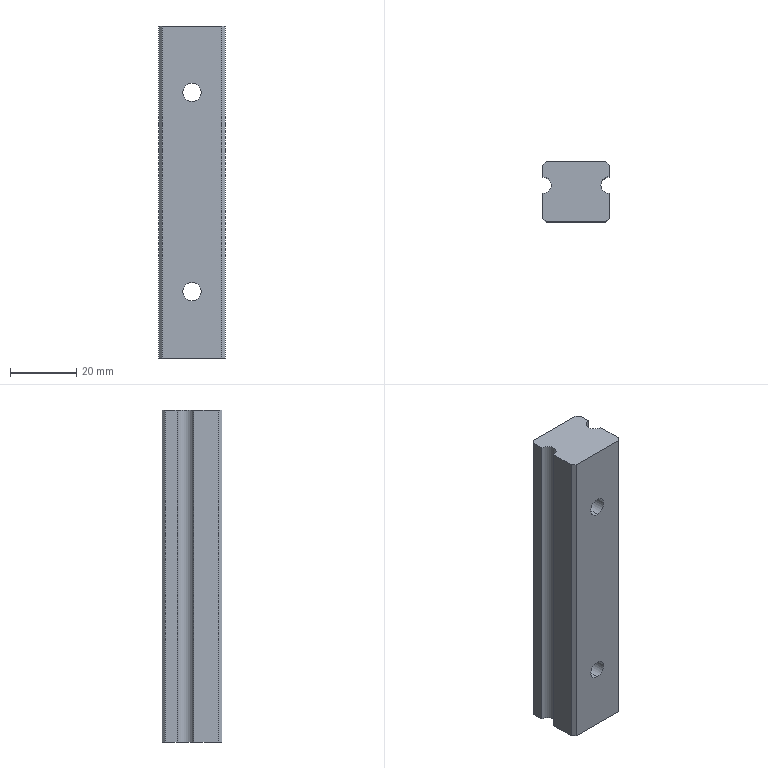Part | SolidWorks | features 3DProfileFeature 1, Extrusion 1, HoleWzd 1 | 1 solid | 25 faces | box 20 x 18 x 100 mm | volume 32357 mm3 | plane 14 | cylinder 11 | commonest cylinder face diameters 5.5 x4 10 x4 5 x3
STEP:
#1=CARTESIAN_POINT('',(10.,12.3,15.));
#2=VERTEX_POINT('',#1);
#3=CARTESIAN_POINT('',(10.,12.3,25.));
#4=VERTEX_POINT('',#3);
#5=CARTESIAN_POINT('',(10.,12.3,20.));
#6=DIRECTION('',(0.,1.,0.));
#7=DIRECTION('',(0.,0.,1.));
#8=AXIS2_PLACEMENT_3D('',#5,#6,#7);
#9=CIRCLE('',#8,5.);
#10=EDGE_CURVE('',#2,#4,#9,.T.);
#11=ORIENTED_EDGE('',*,*,#10,.F.);
#12=CARTESIAN_POINT('',(10.,18.,15.));
#13=VERTEX_POINT('',#12);
#14=CARTESIAN_POINT('',(10.,18.,15.));
#15=DIRECTION('',(0.,1.,0.));
#16=VECTOR('',#15,1000.);
#17=LINE('',#14,#16);
#18=EDGE_CURVE('',#2,#13,#17,.T.);
#19=ORIENTED_EDGE('',*,*,#18,.T.);
#20=CARTESIAN_POINT('',(10.,18.,25.));
#21=VERTEX_POINT('',#20);
#22=CARTESIAN_POINT('',(10.,18.,20.));
#23=DIRECTION('',(0.,1.,0.));
#24=DIRECTION('',(0.,0.,1.));
#25=AXIS2_PLACEMENT_3D('',#22,#23,#24);
#26=CIRCLE('',#25,5.);
#27=EDGE_CURVE('',#13,#21,#26,.T.);
#28=ORIENTED_EDGE('',*,*,#27,.T.);
#29=CARTESIAN_POINT('',(10.,18.,25.));
#30=DIRECTION('',(0.,1.,0.));
#31=VECTOR('',#30,1000.);
#32=LINE('',#29,#31);
#33=EDGE_CURVE('',#4,#21,#32,.T.);
#34=ORIENTED_EDGE('',*,*,#33,.F.);
#35=EDGE_LOOP('',(#11,#19,#28,#34));
#36=FACE_OUTER_BOUND('',#35,.T.);
#37=CARTESIAN_POINT('',(10.,18.,20.));
#38=DIRECTION('',(0.,1.,0.));
#39=DIRECTION('',(0.,0.,1.));
#40=AXIS2_PLACEMENT_3D('',#37,#38,#39);
#41=CYLINDRICAL_SURFACE('',#40,5.);
#42=ADVANCED_FACE('',(#36),#41,.F.);
#43=CARTESIAN_POINT('',(10.,0.,17.25));
#44=VERTEX_POINT('',#43);
#45=CARTESIAN_POINT('',(10.,0.,22.75));
#46=VERTEX_POINT('',#45);
#47=CARTESIAN_POINT('',(10.,0.,20.));
#48=DIRECTION('',(0.,1.,0.));
#49=DIRECTION('',(0.,0.,1.));
#50=AXIS2_PLACEMENT_3D('',#47,#48,#49);
#51=CIRCLE('',#50,2.75);
#52=EDGE_CURVE('',#44,#46,#51,.T.);
#53=ORIENTED_EDGE('',*,*,#52,.F.);
#54=CARTESIAN_POINT('',(10.,12.3,17.25));
#55=VERTEX_POINT('',#54);
#56=CARTESIAN_POINT('',(10.,18.,17.25));
#57=DIRECTION('',(0.,1.,0.));
#58=VECTOR('',#57,1000.);
#59=LINE('',#56,#58);
#60=EDGE_CURVE('',#44,#55,#59,.T.);
#61=ORIENTED_EDGE('',*,*,#60,.T.);
#62=CARTESIAN_POINT('',(10.,12.3,22.75));
#63=VERTEX_POINT('',#62);
#64=CARTESIAN_POINT('',(10.,12.3,20.));
#65=DIRECTION('',(0.,1.,0.));
#66=DIRECTION('',(0.,0.,1.));
#67=AXIS2_PLACEMENT_3D('',#64,#65,#66);
#68=CIRCLE('',#67,2.75);
#69=EDGE_CURVE('',#55,#63,#68,.T.);
#70=ORIENTED_EDGE('',*,*,#69,.T.);
#71=CARTESIAN_POINT('',(10.,18.,22.75));
#72=DIRECTION('',(0.,1.,0.));
#73=VECTOR('',#72,1000.);
#74=LINE('',#71,#73);
#75=EDGE_CURVE('',#46,#63,#74,.T.);
#76=ORIENTED_EDGE('',*,*,#75,.F.);
#77=EDGE_LOOP('',(#53,#61,#70,#76));
#78=FACE_OUTER_BOUND('',#77,.T.);
#79=CARTESIAN_POINT('',(10.,18.,20.));
#80=DIRECTION('',(0.,1.,0.));
#81=DIRECTION('',(0.,0.,1.));
#82=AXIS2_PLACEMENT_3D('',#79,#80,#81);
#83=CYLINDRICAL_SURFACE('',#82,2.75);
#84=ADVANCED_FACE('',(#78),#83,.F.);
#85=CARTESIAN_POINT('',(10.,12.3,75.));
#86=VERTEX_POINT('',#85);
#87=CARTESIAN_POINT('',(10.,12.3,85.));
#88=VERTEX_POINT('',#87);
#89=CARTESIAN_POINT('',(10.,12.3,80.));
#90=DIRECTION('',(0.,1.,0.));
#91=DIRECTION('',(0.,0.,1.));
#92=AXIS2_PLACEMENT_3D('',#89,#90,#91);
#93=CIRCLE('',#92,5.);
#94=EDGE_CURVE('',#86,#88,#93,.T.);
#95=ORIENTED_EDGE('',*,*,#94,.F.);
#96=CARTESIAN_POINT('',(10.,18.,75.));
#97=VERTEX_POINT('',#96);
#98=CARTESIAN_POINT('',(10.,18.,75.));
#99=DIRECTION('',(0.,1.,0.));
#100=VECTOR('',#99,1000.);
#101=LINE('',#98,#100);
#102=EDGE_CURVE('',#86,#97,#101,.T.);
#103=ORIENTED_EDGE('',*,*,#102,.T.);
#104=CARTESIAN_POINT('',(10.,18.,85.));
#105=VERTEX_POINT('',#104);
#106=CARTESIAN_POINT('',(10.,18.,80.));
#107=DIRECTION('',(0.,1.,0.));
#108=DIRECTION('',(0.,0.,1.));
#109=AXIS2_PLACEMENT_3D('',#106,#107,#108);
#110=CIRCLE('',#109,5.);
#111=EDGE_CURVE('',#97,#105,#110,.T.);
#112=ORIENTED_EDGE('',*,*,#111,.T.);
#113=CARTESIAN_POINT('',(10.,18.,85.));
#114=DIRECTION('',(0.,1.,0.));
#115=VECTOR('',#114,1000.);
#116=LINE('',#113,#115);
#117=EDGE_CURVE('',#88,#105,#116,.T.);
#118=ORIENTED_EDGE('',*,*,#117,.F.);
#119=EDGE_LOOP('',(#95,#103,#112,#118));
#120=FACE_OUTER_BOUND('',#119,.T.);
#121=CARTESIAN_POINT('',(10.,18.,80.));
#122=DIRECTION('',(0.,1.,0.));
#123=DIRECTION('',(0.,0.,1.));
#124=AXIS2_PLACEMENT_3D('',#121,#122,#123);
#125=CYLINDRICAL_SURFACE('',#124,5.);
#126=ADVANCED_FACE('',(#120),#125,.F.);
#127=CARTESIAN_POINT('',(10.,0.,77.25));
#128=VERTEX_POINT('',#127);
#129=CARTESIAN_POINT('',(10.,0.,82.75));
#130=VERTEX_POINT('',#129);
#131=CARTESIAN_POINT('',(10.,0.,80.));
#132=DIRECTION('',(0.,1.,0.));
#133=DIRECTION('',(0.,0.,1.));
#134=AXIS2_PLACEMENT_3D('',#131,#132,#133);
#135=CIRCLE('',#134,2.75);
#136=EDGE_CURVE('',#128,#130,#135,.T.);
#137=ORIENTED_EDGE('',*,*,#136,.F.);
#138=CARTESIAN_POINT('',(10.,12.3,77.25));
#139=VERTEX_POINT('',#138);
#140=CARTESIAN_POINT('',(10.,18.,77.25));
#141=DIRECTION('',(0.,1.,0.));
#142=VECTOR('',#141,1000.);
#143=LINE('',#140,#142);
#144=EDGE_CURVE('',#128,#139,#143,.T.);
#145=ORIENTED_EDGE('',*,*,#144,.T.);
#146=CARTESIAN_POINT('',(10.,12.3,82.75));
#147=VERTEX_POINT('',#146);
#148=CARTESIAN_POINT('',(10.,12.3,80.));
#149=DIRECTION('',(0.,1.,0.));
#150=DIRECTION('',(0.,0.,1.));
#151=AXIS2_PLACEMENT_3D('',#148,#149,#150);
#152=CIRCLE('',#151,2.75);
#153=EDGE_CURVE('',#139,#147,#152,.T.);
#154=ORIENTED_EDGE('',*,*,#153,.T.);
#155=CARTESIAN_POINT('',(10.,18.,82.75));
#156=DIRECTION('',(0.,1.,0.));
#157=VECTOR('',#156,1000.);
#158=LINE('',#155,#157);
#159=EDGE_CURVE('',#130,#147,#158,.T.);
#160=ORIENTED_EDGE('',*,*,#159,.F.);
#161=EDGE_LOOP('',(#137,#145,#154,#160));
#162=FACE_OUTER_BOUND('',#161,.T.);
#163=CARTESIAN_POINT('',(10.,18.,80.));
#164=DIRECTION('',(0.,1.,0.));
#165=DIRECTION('',(0.,0.,1.));
#166=AXIS2_PLACEMENT_3D('',#163,#164,#165);
#167=CYLINDRICAL_SURFACE('',#166,2.75);
#168=ADVANCED_FACE('',(#162),#167,.F.);
#169=CARTESIAN_POINT('',(17.5,11.,100.));
#170=VERTEX_POINT('',#169);
#171=CARTESIAN_POINT('',(20.,13.5,100.));
#172=VERTEX_POINT('',#171);
#173=CARTESIAN_POINT('',(20.,11.,100.));
#174=DIRECTION('',(0.,0.,-1.));
#175=DIRECTION('',(1.,0.,0.));
#176=AXIS2_PLACEMENT_3D('',#173,#174,#175);
#177=CIRCLE('',#176,2.5);
#178=EDGE_CURVE('',#170,#172,#177,.T.);
#179=ORIENTED_EDGE('',*,*,#178,.F.);
#180=CARTESIAN_POINT('',(17.5,11.,0.));
#181=VERTEX_POINT('',#180);
#182=CARTESIAN_POINT('',(17.5,11.,100.));
#183=DIRECTION('',(0.,0.,-1.));
#184=VECTOR('',#183,1000.);
#185=LINE('',#182,#184);
#186=EDGE_CURVE('',#170,#181,#185,.T.);
#187=ORIENTED_EDGE('',*,*,#186,.T.);
#188=CARTESIAN_POINT('',(20.,13.5,0.));
#189=VERTEX_POINT('',#188);
#190=CARTESIAN_POINT('',(20.,11.,0.));
#191=DIRECTION('',(0.,0.,-1.));
#192=DIRECTION('',(1.,0.,0.));
#193=AXIS2_PLACEMENT_3D('',#190,#191,#192);
#194=CIRCLE('',#193,2.5);
#195=EDGE_CURVE('',#181,#189,#194,.T.);
#196=ORIENTED_EDGE('',*,*,#195,.T.);
#197=CARTESIAN_POINT('',(20.,13.5,100.));
#198=DIRECTION('',(0.,0.,-1.));
#199=VECTOR('',#198,1000.);
#200=LINE('',#197,#199);
#201=EDGE_CURVE('',#172,#189,#200,.T.);
#202=ORIENTED_EDGE('',*,*,#201,.F.);
#203=EDGE_LOOP('',(#179,#187,#196,#202));
#204=FACE_OUTER_BOUND('',#203,.T.);
#205=CARTESIAN_POINT('',(20.,11.,100.));
#206=DIRECTION('',(0.,0.,-1.));
#207=DIRECTION('',(-1.,0.,0.));
#208=AXIS2_PLACEMENT_3D('',#205,#206,#207);
#209=CYLINDRICAL_SURFACE('',#208,2.5);
#210=ADVANCED_FACE('',(#204),#209,.F.);
#211=ORIENTED_EDGE('',*,*,#186,.F.);
#212=CARTESIAN_POINT('',(20.,8.5,100.));
#213=VERTEX_POINT('',#212);
#214=CARTESIAN_POINT('',(20.,11.,100.));
#215=DIRECTION('',(0.,0.,-1.));
#216=DIRECTION('',(1.,0.,0.));
#217=AXIS2_PLACEMENT_3D('',#214,#215,#216);
#218=CIRCLE('',#217,2.5);
#219=EDGE_CURVE('',#213,#170,#218,.T.);
#220=ORIENTED_EDGE('',*,*,#219,.F.);
#221=CARTESIAN_POINT('',(20.,8.5,0.));
#222=VERTEX_POINT('',#221);
#223=CARTESIAN_POINT('',(20.,8.5,100.));
#224=DIRECTION('',(0.,0.,-1.));
#225=VECTOR('',#224,1000.);
#226=LINE('',#223,#225);
#227=EDGE_CURVE('',#213,#222,#226,.T.);
#228=ORIENTED_EDGE('',*,*,#227,.T.);
#229=CARTESIAN_POINT('',(20.,11.,0.));
#230=DIRECTION('',(0.,0.,-1.));
#231=DIRECTION('',(1.,0.,0.));
#232=AXIS2_PLACEMENT_3D('',#229,#230,#231);
#233=CIRCLE('',#232,2.5);
#234=EDGE_CURVE('',#222,#181,#233,.T.);
#235=ORIENTED_EDGE('',*,*,#234,.T.);
#236=EDGE_LOOP('',(#211,#220,#228,#235));
#237=FACE_OUTER_BOUND('',#236,.T.);
#238=CARTESIAN_POINT('',(20.,11.,100.));
#239=DIRECTION('',(0.,0.,-1.));
#240=DIRECTION('',(-1.,0.,0.));
#241=AXIS2_PLACEMENT_3D('',#238,#239,#240);
#242=CYLINDRICAL_SURFACE('',#241,2.5);
#243=ADVANCED_FACE('',(#237),#242,.F.);
#244=CARTESIAN_POINT('',(20.,17.,0.));
#245=VERTEX_POINT('',#244);
#246=CARTESIAN_POINT('',(20.,13.5,0.));
#247=DIRECTION('',(0.,1.,0.));
#248=VECTOR('',#247,1000.);
#249=LINE('',#246,#248);
#250=EDGE_CURVE('',#189,#245,#249,.T.);
#251=ORIENTED_EDGE('',*,*,#250,.T.);
#252=CARTESIAN_POINT('',(20.,17.,100.));
#253=VERTEX_POINT('',#252);
#254=CARTESIAN_POINT('',(20.,17.,100.));
#255=DIRECTION('',(0.,0.,-1.));
#256=VECTOR('',#255,1000.);
#257=LINE('',#254,#256);
#258=EDGE_CURVE('',#253,#245,#257,.T.);
#259=ORIENTED_EDGE('',*,*,#258,.F.);
#260=CARTESIAN_POINT('',(20.,13.5,100.));
#261=DIRECTION('',(0.,1.,0.));
#262=VECTOR('',#261,1000.);
#263=LINE('',#260,#262);
#264=EDGE_CURVE('',#172,#253,#263,.T.);
#265=ORIENTED_EDGE('',*,*,#264,.F.);
#266=ORIENTED_EDGE('',*,*,#201,.T.);
#267=EDGE_LOOP('',(#251,#259,#265,#266));
#268=FACE_OUTER_BOUND('',#267,.T.);
#269=CARTESIAN_POINT('',(20.,13.5,100.));
#270=DIRECTION('',(-1.,0.,0.));
#271=DIRECTION('',(0.,0.,1.));
#272=AXIS2_PLACEMENT_3D('',#269,#270,#271);
#273=PLANE('',#272);
#274=ADVANCED_FACE('',(#268),#273,.F.);
#275=CARTESIAN_POINT('',(19.,18.,0.));
#276=VERTEX_POINT('',#275);
#277=CARTESIAN_POINT('',(19.,18.,0.));
#278=DIRECTION('',(-0.7071,0.7071,0.));
#279=VECTOR('',#278,1000.);
#280=LINE('',#277,#279);
#281=EDGE_CURVE('',#245,#276,#280,.T.);
#282=ORIENTED_EDGE('',*,*,#281,.T.);
#283=CARTESIAN_POINT('',(19.,18.,100.));
#284=VERTEX_POINT('',#283);
#285=CARTESIAN_POINT('',(19.,18.,100.));
#286=DIRECTION('',(0.,0.,-1.));
#287=VECTOR('',#286,1000.);
#288=LINE('',#285,#287);
#289=EDGE_CURVE('',#284,#276,#288,.T.);
#290=ORIENTED_EDGE('',*,*,#289,.F.);
#291=CARTESIAN_POINT('',(19.,18.,100.));
#292=DIRECTION('',(-0.7071,0.7071,0.));
#293=VECTOR('',#292,1000.);
#294=LINE('',#291,#293);
#295=EDGE_CURVE('',#253,#284,#294,.T.);
#296=ORIENTED_EDGE('',*,*,#295,.F.);
#297=ORIENTED_EDGE('',*,*,#258,.T.);
#298=EDGE_LOOP('',(#282,#290,#296,#297));
#299=FACE_OUTER_BOUND('',#298,.T.);
#300=CARTESIAN_POINT('',(19.,18.,100.));
#301=DIRECTION('',(-0.7071,-0.7071,0.));
#302=DIRECTION('',(0.7071,-0.7071,0.));
#303=AXIS2_PLACEMENT_3D('',#300,#301,#302);
#304=PLANE('',#303);
#305=ADVANCED_FACE('',(#299),#304,.F.);
#306=CARTESIAN_POINT('',(10.,18.,20.));
#307=DIRECTION('',(0.,1.,0.));
#308=DIRECTION('',(0.,0.,1.));
#309=AXIS2_PLACEMENT_3D('',#306,#307,#308);
#310=CIRCLE('',#309,5.);
#311=EDGE_CURVE('',#21,#13,#310,.T.);
#312=ORIENTED_EDGE('',*,*,#311,.F.);
#313=ORIENTED_EDGE('',*,*,#27,.F.);
#314=EDGE_LOOP('',(#312,#313));
#315=FACE_BOUND('',#314,.T.);
#316=CARTESIAN_POINT('',(10.,18.,80.));
#317=DIRECTION('',(0.,1.,0.));
#318=DIRECTION('',(0.,0.,1.));
#319=AXIS2_PLACEMENT_3D('',#316,#317,#318);
#320=CIRCLE('',#319,5.);
#321=EDGE_CURVE('',#105,#97,#320,.T.);
#322=ORIENTED_EDGE('',*,*,#321,.F.);
#323=ORIENTED_EDGE('',*,*,#111,.F.);
#324=EDGE_LOOP('',(#322,#323));
#325=FACE_BOUND('',#324,.T.);
#326=CARTESIAN_POINT('',(1.,18.,0.));
#327=VERTEX_POINT('',#326);
#328=CARTESIAN_POINT('',(1.,18.,0.));
#329=DIRECTION('',(-1.,0.,0.));
#330=VECTOR('',#329,1000.);
#331=LINE('',#328,#330);
#332=EDGE_CURVE('',#276,#327,#331,.T.);
#333=ORIENTED_EDGE('',*,*,#332,.T.);
#334=CARTESIAN_POINT('',(1.,18.,100.));
#335=VERTEX_POINT('',#334);
#336=CARTESIAN_POINT('',(1.,18.,100.));
#337=DIRECTION('',(0.,0.,-1.));
#338=VECTOR('',#337,1000.);
#339=LINE('',#336,#338);
#340=EDGE_CURVE('',#335,#327,#339,.T.);
#341=ORIENTED_EDGE('',*,*,#340,.F.);
#342=CARTESIAN_POINT('',(1.,18.,100.));
#343=DIRECTION('',(-1.,0.,0.));
#344=VECTOR('',#343,1000.);
#345=LINE('',#342,#344);
#346=EDGE_CURVE('',#284,#335,#345,.T.);
#347=ORIENTED_EDGE('',*,*,#346,.F.);
#348=ORIENTED_EDGE('',*,*,#289,.T.);
#349=EDGE_LOOP('',(#333,#341,#347,#348));
#350=FACE_OUTER_BOUND('',#349,.T.);
#351=CARTESIAN_POINT('',(1.,18.,100.));
#352=DIRECTION('',(0.,-1.,0.));
#353=DIRECTION('',(0.,0.,-1.));
#354=AXIS2_PLACEMENT_3D('',#351,#352,#353);
#355=PLANE('',#354);
#356=ADVANCED_FACE('',(#315,#325,#350),#355,.F.);
#357=CARTESIAN_POINT('',(0.,17.,0.));
#358=VERTEX_POINT('',#357);
#359=CARTESIAN_POINT('',(0.,17.,0.));
#360=DIRECTION('',(-0.7071,-0.7071,0.));
#361=VECTOR('',#360,1000.);
#362=LINE('',#359,#361);
#363=EDGE_CURVE('',#327,#358,#362,.T.);
#364=ORIENTED_EDGE('',*,*,#363,.T.);
#365=CARTESIAN_POINT('',(0.,17.,100.));
#366=VERTEX_POINT('',#365);
#367=CARTESIAN_POINT('',(0.,17.,100.));
#368=DIRECTION('',(0.,0.,-1.));
#369=VECTOR('',#368,1000.);
#370=LINE('',#367,#369);
#371=EDGE_CURVE('',#366,#358,#370,.T.);
#372=ORIENTED_EDGE('',*,*,#371,.F.);
#373=CARTESIAN_POINT('',(0.,17.,100.));
#374=DIRECTION('',(-0.7071,-0.7071,0.));
#375=VECTOR('',#374,1000.);
#376=LINE('',#373,#375);
#377=EDGE_CURVE('',#335,#366,#376,.T.);
#378=ORIENTED_EDGE('',*,*,#377,.F.);
#379=ORIENTED_EDGE('',*,*,#340,.T.);
#380=EDGE_LOOP('',(#364,#372,#378,#379));
#381=FACE_OUTER_BOUND('',#380,.T.);
#382=CARTESIAN_POINT('',(0.,17.,100.));
#383=DIRECTION('',(0.7071,-0.7071,0.));
#384=DIRECTION('',(0.7071,0.7071,0.));
#385=AXIS2_PLACEMENT_3D('',#382,#383,#384);
#386=PLANE('',#385);
#387=ADVANCED_FACE('',(#381),#386,.F.);
#388=CARTESIAN_POINT('',(0.,13.5,0.));
#389=VERTEX_POINT('',#388);
#390=CARTESIAN_POINT('',(0.,13.5,0.));
#391=DIRECTION('',(0.,-1.,0.));
#392=VECTOR('',#391,1000.);
#393=LINE('',#390,#392);
#394=EDGE_CURVE('',#358,#389,#393,.T.);
#395=ORIENTED_EDGE('',*,*,#394,.T.);
#396=CARTESIAN_POINT('',(0.,13.5,100.));
#397=VERTEX_POINT('',#396);
#398=CARTESIAN_POINT('',(0.,13.5,100.));
#399=DIRECTION('',(0.,0.,-1.));
#400=VECTOR('',#399,1000.);
#401=LINE('',#398,#400);
#402=EDGE_CURVE('',#397,#389,#401,.T.);
#403=ORIENTED_EDGE('',*,*,#402,.F.);
#404=CARTESIAN_POINT('',(0.,13.5,100.));
#405=DIRECTION('',(0.,-1.,0.));
#406=VECTOR('',#405,1000.);
#407=LINE('',#404,#406);
#408=EDGE_CURVE('',#366,#397,#407,.T.);
#409=ORIENTED_EDGE('',*,*,#408,.F.);
#410=ORIENTED_EDGE('',*,*,#371,.T.);
#411=EDGE_LOOP('',(#395,#403,#409,#410));
#412=FACE_OUTER_BOUND('',#411,.T.);
#413=CARTESIAN_POINT('',(0.,13.5,100.));
#414=DIRECTION('',(1.,0.,0.));
#415=DIRECTION('',(0.,0.,-1.));
#416=AXIS2_PLACEMENT_3D('',#413,#414,#415);
#417=PLANE('',#416);
#418=ADVANCED_FACE('',(#412),#417,.F.);
#419=CARTESIAN_POINT('',(0.,8.5,0.));
#420=VERTEX_POINT('',#419);
#421=CARTESIAN_POINT('',(0.,11.,0.));
#422=DIRECTION('',(0.,0.,-1.));
#423=DIRECTION('',(1.,0.,0.));
#424=AXIS2_PLACEMENT_3D('',#421,#422,#423);
#425=CIRCLE('',#424,2.5);
#426=EDGE_CURVE('',#389,#420,#425,.T.);
#427=ORIENTED_EDGE('',*,*,#426,.T.);
#428=CARTESIAN_POINT('',(0.,8.5,100.));
#429=VERTEX_POINT('',#428);
#430=CARTESIAN_POINT('',(0.,8.5,100.));
#431=DIRECTION('',(0.,0.,-1.));
#432=VECTOR('',#431,1000.);
#433=LINE('',#430,#432);
#434=EDGE_CURVE('',#429,#420,#433,.T.);
#435=ORIENTED_EDGE('',*,*,#434,.F.);
#436=CARTESIAN_POINT('',(0.,11.,100.));
#437=DIRECTION('',(0.,0.,-1.));
#438=DIRECTION('',(1.,0.,0.));
#439=AXIS2_PLACEMENT_3D('',#436,#437,#438);
#440=CIRCLE('',#439,2.5);
#441=EDGE_CURVE('',#397,#429,#440,.T.);
#442=ORIENTED_EDGE('',*,*,#441,.F.);
#443=ORIENTED_EDGE('',*,*,#402,.T.);
#444=EDGE_LOOP('',(#427,#435,#442,#443));
#445=FACE_OUTER_BOUND('',#444,.T.);
#446=CARTESIAN_POINT('',(0.,11.,100.));
#447=DIRECTION('',(0.,0.,-1.));
#448=DIRECTION('',(-1.,0.,0.));
#449=AXIS2_PLACEMENT_3D('',#446,#447,#448);
#450=CYLINDRICAL_SURFACE('',#449,2.5);
#451=ADVANCED_FACE('',(#445),#450,.F.);
#452=CARTESIAN_POINT('',(0.,1.,0.));
#453=VERTEX_POINT('',#452);
#454=CARTESIAN_POINT('',(0.,1.,0.));
#455=DIRECTION('',(0.,-1.,0.));
#456=VECTOR('',#455,1000.);
#457=LINE('',#454,#456);
#458=EDGE_CURVE('',#420,#453,#457,.T.);
#459=ORIENTED_EDGE('',*,*,#458,.T.);
#460=CARTESIAN_POINT('',(0.,1.,100.));
#461=VERTEX_POINT('',#460);
#462=CARTESIAN_POINT('',(0.,1.,100.));
#463=DIRECTION('',(0.,0.,-1.));
#464=VECTOR('',#463,1000.);
#465=LINE('',#462,#464);
#466=EDGE_CURVE('',#461,#453,#465,.T.);
#467=ORIENTED_EDGE('',*,*,#466,.F.);
#468=CARTESIAN_POINT('',(0.,1.,100.));
#469=DIRECTION('',(0.,-1.,0.));
#470=VECTOR('',#469,1000.);
#471=LINE('',#468,#470);
#472=EDGE_CURVE('',#429,#461,#471,.T.);
#473=ORIENTED_EDGE('',*,*,#472,.F.);
#474=ORIENTED_EDGE('',*,*,#434,.T.);
#475=EDGE_LOOP('',(#459,#467,#473,#474));
#476=FACE_OUTER_BOUND('',#475,.T.);
#477=CARTESIAN_POINT('',(0.,1.,100.));
#478=DIRECTION('',(1.,0.,0.));
#479=DIRECTION('',(0.,0.,-1.));
#480=AXIS2_PLACEMENT_3D('',#477,#478,#479);
#481=PLANE('',#480);
#482=ADVANCED_FACE('',(#476),#481,.F.);
#483=CARTESIAN_POINT('',(1.,0.,0.));
#484=VERTEX_POINT('',#483);
#485=CARTESIAN_POINT('',(0.,1.,0.));
#486=DIRECTION('',(0.7071,-0.7071,0.));
#487=VECTOR('',#486,1000.);
#488=LINE('',#485,#487);
#489=EDGE_CURVE('',#453,#484,#488,.T.);
#490=ORIENTED_EDGE('',*,*,#489,.T.);
#491=CARTESIAN_POINT('',(1.,0.,100.));
#492=VERTEX_POINT('',#491);
#493=CARTESIAN_POINT('',(1.,0.,100.));
#494=DIRECTION('',(0.,0.,-1.));
#495=VECTOR('',#494,1000.);
#496=LINE('',#493,#495);
#497=EDGE_CURVE('',#492,#484,#496,.T.);
#498=ORIENTED_EDGE('',*,*,#497,.F.);
#499=CARTESIAN_POINT('',(0.,1.,100.));
#500=DIRECTION('',(0.7071,-0.7071,0.));
#501=VECTOR('',#500,1000.);
#502=LINE('',#499,#501);
#503=EDGE_CURVE('',#461,#492,#502,.T.);
#504=ORIENTED_EDGE('',*,*,#503,.F.);
#505=ORIENTED_EDGE('',*,*,#466,.T.);
#506=EDGE_LOOP('',(#490,#498,#504,#505));
#507=FACE_OUTER_BOUND('',#506,.T.);
#508=CARTESIAN_POINT('',(0.,1.,100.));
#509=DIRECTION('',(0.7071,0.7071,0.));
#510=DIRECTION('',(-0.7071,0.7071,0.));
#511=AXIS2_PLACEMENT_3D('',#508,#509,#510);
#512=PLANE('',#511);
#513=ADVANCED_FACE('',(#507),#512,.F.);
#514=CARTESIAN_POINT('',(10.,0.,20.));
#515=DIRECTION('',(0.,1.,0.));
#516=DIRECTION('',(0.,0.,1.));
#517=AXIS2_PLACEMENT_3D('',#514,#515,#516);
#518=CIRCLE('',#517,2.75);
#519=EDGE_CURVE('',#46,#44,#518,.T.);
#520=ORIENTED_EDGE('',*,*,#519,.T.);
#521=ORIENTED_EDGE('',*,*,#52,.T.);
#522=EDGE_LOOP('',(#520,#521));
#523=FACE_BOUND('',#522,.T.);
#524=CARTESIAN_POINT('',(10.,0.,80.));
#525=DIRECTION('',(0.,1.,0.));
#526=DIRECTION('',(0.,0.,1.));
#527=AXIS2_PLACEMENT_3D('',#524,#525,#526);
#528=CIRCLE('',#527,2.75);
#529=EDGE_CURVE('',#130,#128,#528,.T.);
#530=ORIENTED_EDGE('',*,*,#529,.T.);
#531=ORIENTED_EDGE('',*,*,#136,.T.);
#532=EDGE_LOOP('',(#530,#531));
#533=FACE_BOUND('',#532,.T.);
#534=CARTESIAN_POINT('',(19.,0.,0.));
#535=VERTEX_POINT('',#534);
#536=CARTESIAN_POINT('',(1.,0.,0.));
#537=DIRECTION('',(1.,0.,0.));
#538=VECTOR('',#537,1000.);
#539=LINE('',#536,#538);
#540=EDGE_CURVE('',#484,#535,#539,.T.);
#541=ORIENTED_EDGE('',*,*,#540,.T.);
#542=CARTESIAN_POINT('',(19.,0.,100.));
#543=VERTEX_POINT('',#542);
#544=CARTESIAN_POINT('',(19.,0.,100.));
#545=DIRECTION('',(0.,0.,-1.));
#546=VECTOR('',#545,1000.);
#547=LINE('',#544,#546);
#548=EDGE_CURVE('',#543,#535,#547,.T.);
#549=ORIENTED_EDGE('',*,*,#548,.F.);
#550=CARTESIAN_POINT('',(1.,0.,100.));
#551=DIRECTION('',(1.,0.,0.));
#552=VECTOR('',#551,1000.);
#553=LINE('',#550,#552);
#554=EDGE_CURVE('',#492,#543,#553,.T.);
#555=ORIENTED_EDGE('',*,*,#554,.F.);
#556=ORIENTED_EDGE('',*,*,#497,.T.);
#557=EDGE_LOOP('',(#541,#549,#555,#556));
#558=FACE_OUTER_BOUND('',#557,.T.);
#559=CARTESIAN_POINT('',(1.,0.,100.));
#560=DIRECTION('',(0.,1.,0.));
#561=DIRECTION('',(0.,0.,1.));
#562=AXIS2_PLACEMENT_3D('',#559,#560,#561);
#563=PLANE('',#562);
#564=ADVANCED_FACE('',(#523,#533,#558),#563,.F.);
#565=CARTESIAN_POINT('',(20.,1.,0.));
#566=VERTEX_POINT('',#565);
#567=CARTESIAN_POINT('',(19.,0.,0.));
#568=DIRECTION('',(0.7071,0.7071,0.));
#569=VECTOR('',#568,1000.);
#570=LINE('',#567,#569);
#571=EDGE_CURVE('',#535,#566,#570,.T.);
#572=ORIENTED_EDGE('',*,*,#571,.T.);
#573=CARTESIAN_POINT('',(20.,1.,100.));
#574=VERTEX_POINT('',#573);
#575=CARTESIAN_POINT('',(20.,1.,100.));
#576=DIRECTION('',(0.,0.,-1.));
#577=VECTOR('',#576,1000.);
#578=LINE('',#575,#577);
#579=EDGE_CURVE('',#574,#566,#578,.T.);
#580=ORIENTED_EDGE('',*,*,#579,.F.);
#581=CARTESIAN_POINT('',(19.,0.,100.));
#582=DIRECTION('',(0.7071,0.7071,0.));
#583=VECTOR('',#582,1000.);
#584=LINE('',#581,#583);
#585=EDGE_CURVE('',#543,#574,#584,.T.);
#586=ORIENTED_EDGE('',*,*,#585,.F.);
#587=ORIENTED_EDGE('',*,*,#548,.T.);
#588=EDGE_LOOP('',(#572,#580,#586,#587));
#589=FACE_OUTER_BOUND('',#588,.T.);
#590=CARTESIAN_POINT('',(19.,0.,100.));
#591=DIRECTION('',(-0.7071,0.7071,0.));
#592=DIRECTION('',(-0.7071,-0.7071,0.));
#593=AXIS2_PLACEMENT_3D('',#590,#591,#592);
#594=PLANE('',#593);
#595=ADVANCED_FACE('',(#589),#594,.F.);
#596=CARTESIAN_POINT('',(20.,1.,0.));
#597=DIRECTION('',(0.,1.,0.));
#598=VECTOR('',#597,1000.);
#599=LINE('',#596,#598);
#600=EDGE_CURVE('',#566,#222,#599,.T.);
#601=ORIENTED_EDGE('',*,*,#600,.T.);
#602=ORIENTED_EDGE('',*,*,#227,.F.);
#603=CARTESIAN_POINT('',(20.,1.,100.));
#604=DIRECTION('',(0.,1.,0.));
#605=VECTOR('',#604,1000.);
#606=LINE('',#603,#605);
#607=EDGE_CURVE('',#574,#213,#606,.T.);
#608=ORIENTED_EDGE('',*,*,#607,.F.);
#609=ORIENTED_EDGE('',*,*,#579,.T.);
#610=EDGE_LOOP('',(#601,#602,#608,#609));
#611=FACE_OUTER_BOUND('',#610,.T.);
#612=CARTESIAN_POINT('',(20.,1.,100.));
#613=DIRECTION('',(-1.,0.,0.));
#614=DIRECTION('',(0.,0.,1.));
#615=AXIS2_PLACEMENT_3D('',#612,#613,#614);
#616=PLANE('',#615);
#617=ADVANCED_FACE('',(#611),#616,.F.);
#618=ORIENTED_EDGE('',*,*,#219,.T.);
#619=ORIENTED_EDGE('',*,*,#178,.T.);
#620=ORIENTED_EDGE('',*,*,#264,.T.);
#621=ORIENTED_EDGE('',*,*,#295,.T.);
#622=ORIENTED_EDGE('',*,*,#346,.T.);
#623=ORIENTED_EDGE('',*,*,#377,.T.);
#624=ORIENTED_EDGE('',*,*,#408,.T.);
#625=ORIENTED_EDGE('',*,*,#441,.T.);
#626=ORIENTED_EDGE('',*,*,#472,.T.);
#627=ORIENTED_EDGE('',*,*,#503,.T.);
#628=ORIENTED_EDGE('',*,*,#554,.T.);
#629=ORIENTED_EDGE('',*,*,#585,.T.);
#630=ORIENTED_EDGE('',*,*,#607,.T.);
#631=EDGE_LOOP('',(#618,#619,#620,#621,#622,#623,#624,#625,#626,#627,#628,#629,#630));
#632=FACE_OUTER_BOUND('',#631,.T.);
#633=CARTESIAN_POINT('',(20.,11.,100.));
#634=DIRECTION('',(0.,0.,1.));
#635=DIRECTION('',(1.,0.,0.));
#636=AXIS2_PLACEMENT_3D('',#633,#634,#635);
#637=PLANE('',#636);
#638=ADVANCED_FACE('',(#632),#637,.T.);
#639=ORIENTED_EDGE('',*,*,#234,.F.);
#640=ORIENTED_EDGE('',*,*,#600,.F.);
#641=ORIENTED_EDGE('',*,*,#571,.F.);
#642=ORIENTED_EDGE('',*,*,#540,.F.);
#643=ORIENTED_EDGE('',*,*,#489,.F.);
#644=ORIENTED_EDGE('',*,*,#458,.F.);
#645=ORIENTED_EDGE('',*,*,#426,.F.);
#646=ORIENTED_EDGE('',*,*,#394,.F.);
#647=ORIENTED_EDGE('',*,*,#363,.F.);
#648=ORIENTED_EDGE('',*,*,#332,.F.);
#649=ORIENTED_EDGE('',*,*,#281,.F.);
#650=ORIENTED_EDGE('',*,*,#250,.F.);
#651=ORIENTED_EDGE('',*,*,#195,.F.);
#652=EDGE_LOOP('',(#639,#640,#641,#642,#643,#644,#645,#646,#647,#648,#649,#650,#651));
#653=FACE_OUTER_BOUND('',#652,.T.);
#654=CARTESIAN_POINT('',(20.,11.,0.));
#655=DIRECTION('',(0.,0.,1.));
#656=DIRECTION('',(1.,0.,0.));
#657=AXIS2_PLACEMENT_3D('',#654,#655,#656);
#658=PLANE('',#657);
#659=ADVANCED_FACE('',(#653),#658,.F.);
#660=ORIENTED_EDGE('',*,*,#144,.F.);
#661=ORIENTED_EDGE('',*,*,#529,.F.);
#662=ORIENTED_EDGE('',*,*,#159,.T.);
#663=CARTESIAN_POINT('',(10.,12.3,80.));
#664=DIRECTION('',(0.,1.,0.));
#665=DIRECTION('',(0.,0.,1.));
#666=AXIS2_PLACEMENT_3D('',#663,#664,#665);
#667=CIRCLE('',#666,2.75);
#668=EDGE_CURVE('',#147,#139,#667,.T.);
#669=ORIENTED_EDGE('',*,*,#668,.T.);
#670=EDGE_LOOP('',(#660,#661,#662,#669));
#671=FACE_OUTER_BOUND('',#670,.T.);
#672=CARTESIAN_POINT('',(10.,18.,80.));
#673=DIRECTION('',(0.,1.,0.));
#674=DIRECTION('',(0.,0.,1.));
#675=AXIS2_PLACEMENT_3D('',#672,#673,#674);
#676=CYLINDRICAL_SURFACE('',#675,2.75);
#677=ADVANCED_FACE('',(#671),#676,.F.);
#678=ORIENTED_EDGE('',*,*,#668,.F.);
#679=ORIENTED_EDGE('',*,*,#153,.F.);
#680=EDGE_LOOP('',(#678,#679));
#681=FACE_BOUND('',#680,.T.);
#682=CARTESIAN_POINT('',(10.,12.3,80.));
#683=DIRECTION('',(0.,1.,0.));
#684=DIRECTION('',(0.,0.,1.));
#685=AXIS2_PLACEMENT_3D('',#682,#683,#684);
#686=CIRCLE('',#685,5.);
#687=EDGE_CURVE('',#88,#86,#686,.T.);
#688=ORIENTED_EDGE('',*,*,#687,.T.);
#689=ORIENTED_EDGE('',*,*,#94,.T.);
#690=EDGE_LOOP('',(#688,#689));
#691=FACE_OUTER_BOUND('',#690,.T.);
#692=CARTESIAN_POINT('',(12.75,12.3,80.));
#693=DIRECTION('',(0.,-1.,0.));
#694=DIRECTION('',(0.,0.,-1.));
#695=AXIS2_PLACEMENT_3D('',#692,#693,#694);
#696=PLANE('',#695);
#697=ADVANCED_FACE('',(#681,#691),#696,.F.);
#698=ORIENTED_EDGE('',*,*,#102,.F.);
#699=ORIENTED_EDGE('',*,*,#687,.F.);
#700=ORIENTED_EDGE('',*,*,#117,.T.);
#701=ORIENTED_EDGE('',*,*,#321,.T.);
#702=EDGE_LOOP('',(#698,#699,#700,#701));
#703=FACE_OUTER_BOUND('',#702,.T.);
#704=CARTESIAN_POINT('',(10.,18.,80.));
#705=DIRECTION('',(0.,1.,0.));
#706=DIRECTION('',(0.,0.,1.));
#707=AXIS2_PLACEMENT_3D('',#704,#705,#706);
#708=CYLINDRICAL_SURFACE('',#707,5.);
#709=ADVANCED_FACE('',(#703),#708,.F.);
#710=ORIENTED_EDGE('',*,*,#60,.F.);
#711=ORIENTED_EDGE('',*,*,#519,.F.);
#712=ORIENTED_EDGE('',*,*,#75,.T.);
#713=CARTESIAN_POINT('',(10.,12.3,20.));
#714=DIRECTION('',(0.,1.,0.));
#715=DIRECTION('',(0.,0.,1.));
#716=AXIS2_PLACEMENT_3D('',#713,#714,#715);
#717=CIRCLE('',#716,2.75);
#718=EDGE_CURVE('',#63,#55,#717,.T.);
#719=ORIENTED_EDGE('',*,*,#718,.T.);
#720=EDGE_LOOP('',(#710,#711,#712,#719));
#721=FACE_OUTER_BOUND('',#720,.T.);
#722=CARTESIAN_POINT('',(10.,18.,20.));
#723=DIRECTION('',(0.,1.,0.));
#724=DIRECTION('',(0.,0.,1.));
#725=AXIS2_PLACEMENT_3D('',#722,#723,#724);
#726=CYLINDRICAL_SURFACE('',#725,2.75);
#727=ADVANCED_FACE('',(#721),#726,.F.);
#728=ORIENTED_EDGE('',*,*,#718,.F.);
#729=ORIENTED_EDGE('',*,*,#69,.F.);
#730=EDGE_LOOP('',(#728,#729));
#731=FACE_BOUND('',#730,.T.);
#732=CARTESIAN_POINT('',(10.,12.3,20.));
#733=DIRECTION('',(0.,1.,0.));
#734=DIRECTION('',(0.,0.,1.));
#735=AXIS2_PLACEMENT_3D('',#732,#733,#734);
#736=CIRCLE('',#735,5.);
#737=EDGE_CURVE('',#4,#2,#736,.T.);
#738=ORIENTED_EDGE('',*,*,#737,.T.);
#739=ORIENTED_EDGE('',*,*,#10,.T.);
#740=EDGE_LOOP('',(#738,#739));
#741=FACE_OUTER_BOUND('',#740,.T.);
#742=CARTESIAN_POINT('',(12.75,12.3,20.));
#743=DIRECTION('',(0.,-1.,0.));
#744=DIRECTION('',(0.,0.,-1.));
#745=AXIS2_PLACEMENT_3D('',#742,#743,#744);
#746=PLANE('',#745);
#747=ADVANCED_FACE('',(#731,#741),#746,.F.);
#748=ORIENTED_EDGE('',*,*,#18,.F.);
#749=ORIENTED_EDGE('',*,*,#737,.F.);
#750=ORIENTED_EDGE('',*,*,#33,.T.);
#751=ORIENTED_EDGE('',*,*,#311,.T.);
#752=EDGE_LOOP('',(#748,#749,#750,#751));
#753=FACE_OUTER_BOUND('',#752,.T.);
#754=CARTESIAN_POINT('',(10.,18.,20.));
#755=DIRECTION('',(0.,1.,0.));
#756=DIRECTION('',(0.,0.,1.));
#757=AXIS2_PLACEMENT_3D('',#754,#755,#756);
#758=CYLINDRICAL_SURFACE('',#757,5.);
#759=ADVANCED_FACE('',(#753),#758,.F.);
#760=CLOSED_SHELL('',(#42,#84,#126,#168,#210,#243,#274,#305,#356,#387,#418,#451,#482,#513,#564,#595,#617,#638,#659,#677,#697,#709,#727,#747,#759));
#761=MANIFOLD_SOLID_BREP('',#760);
#762=CARTESIAN_POINT('',(0.,0.,0.));
#763=DIRECTION('',(0.,0.,1.));
#764=DIRECTION('',(1.,0.,0.));
#765=AXIS2_PLACEMENT_3D('',#762,#763,#764);
#766=(LENGTH_UNIT()NAMED_UNIT(*)SI_UNIT(.MILLI.,.METRE.));
#767=UNCERTAINTY_MEASURE_WITH_UNIT(LENGTH_MEASURE(0.00001),#766,'','');
#768=(NAMED_UNIT(*)PLANE_ANGLE_UNIT()SI_UNIT($,.RADIAN.));
#769=(NAMED_UNIT(*)SI_UNIT($,.STERADIAN.)SOLID_ANGLE_UNIT());
#770=(GEOMETRIC_REPRESENTATION_CONTEXT(3)GLOBAL_UNCERTAINTY_ASSIGNED_CONTEXT((#767))GLOBAL_UNIT_ASSIGNED_CONTEXT((#766,#768,#769))REPRESENTATION_CONTEXT('',''));
#771=ADVANCED_BREP_SHAPE_REPRESENTATION('',(#761,#765),#770);